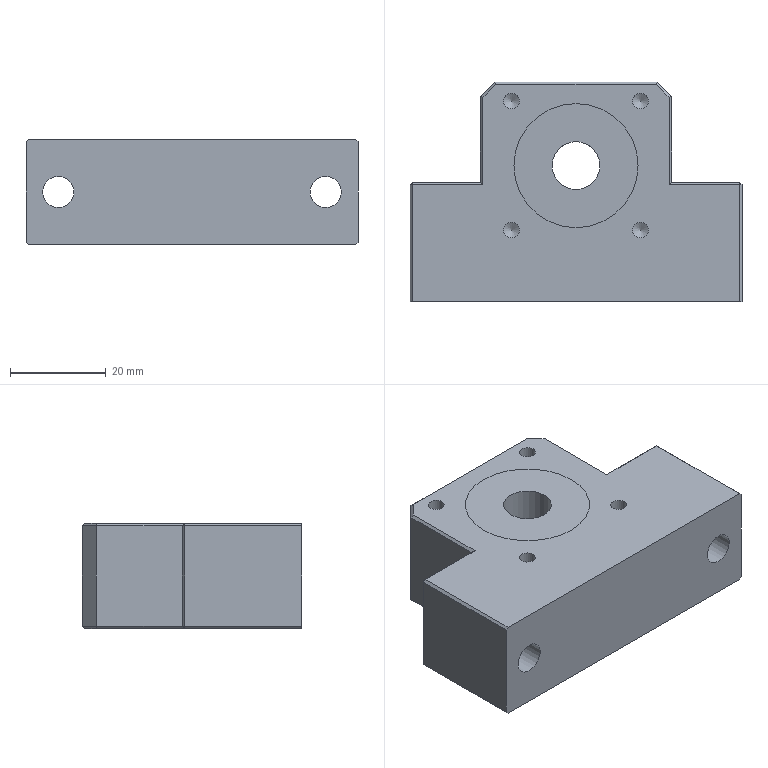Part | STEP file | 2 solids | 55 faces | box 69.5 x 46 x 22 mm | volume 45024 mm3 | plane 40 | cylinder 11 | cone 4 | commonest cylinder face diameters 3.3 x4 10 x3 6.5 x2 26 x2